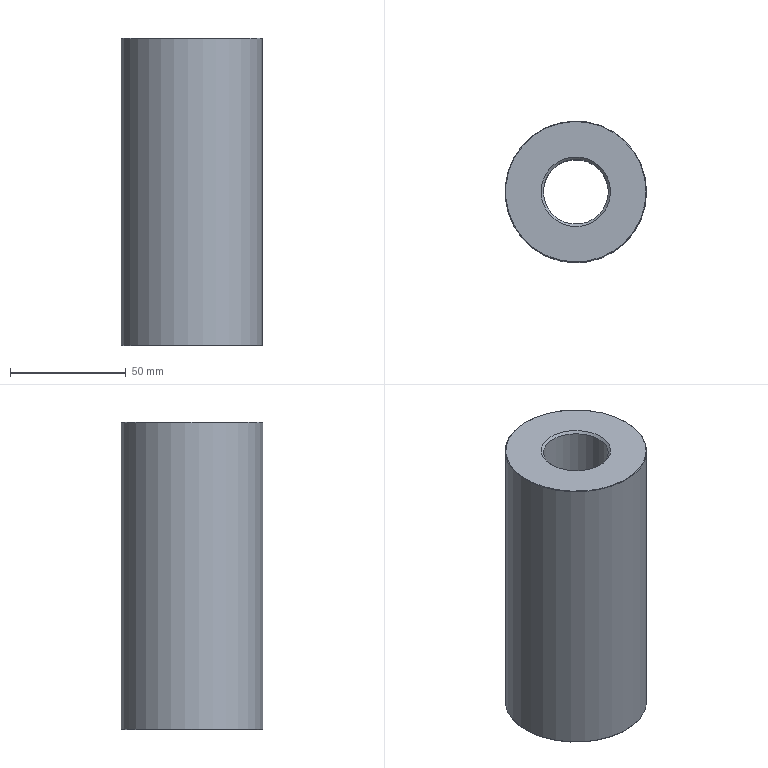Part | NX | features DATUM_CSYS 2, BLEND 1, CHAMFER 1, EXTRUDE 1, SKETCH 1 | 1 solid | 8 faces | box 61 x 61 x 132.5 mm | volume 305546 mm3 | cylinder 2 | plane 2 | cone 2 | torus 2 | commonest cylinder face diameters 28 x1 61 x1
STEP:
#1=CARTESIAN_POINT('',(30.5,0.,0.2));
#2=VERTEX_POINT('',#1);
#3=CARTESIAN_POINT('',(0.,0.,0.2));
#4=DIRECTION('',(0.,0.,1.));
#5=DIRECTION('',(1.,0.,0.));
#6=AXIS2_PLACEMENT_3D('',#3,#4,#5);
#7=CIRCLE('',#6,30.5);
#8=EDGE_CURVE('',#2,#2,#7,.T.);
#9=ORIENTED_EDGE('',*,*,#8,.T.);
#10=EDGE_LOOP('',(#9));
#11=FACE_BOUND('',#10,.T.);
#12=CARTESIAN_POINT('',(30.5,0.,132.3));
#13=VERTEX_POINT('',#12);
#14=CARTESIAN_POINT('',(0.,0.,132.3));
#15=DIRECTION('',(0.,0.,1.));
#16=DIRECTION('',(1.,0.,0.));
#17=AXIS2_PLACEMENT_3D('',#14,#15,#16);
#18=CIRCLE('',#17,30.5);
#19=EDGE_CURVE('',#13,#13,#18,.F.);
#20=ORIENTED_EDGE('',*,*,#19,.T.);
#21=EDGE_LOOP('',(#20));
#22=FACE_BOUND('',#21,.T.);
#23=CARTESIAN_POINT('',(0.,0.,132.5));
#24=DIRECTION('',(0.,0.,-1.));
#25=DIRECTION('',(-1.,0.,0.));
#26=AXIS2_PLACEMENT_3D('',#23,#24,#25);
#27=CYLINDRICAL_SURFACE('',#26,30.5);
#28=ADVANCED_FACE('',(#11,#22),#27,.T.);
#29=CARTESIAN_POINT('',(14.,0.,1.));
#30=VERTEX_POINT('',#29);
#31=CARTESIAN_POINT('',(0.,0.,1.));
#32=DIRECTION('',(0.,0.,1.));
#33=DIRECTION('',(1.,0.,0.));
#34=AXIS2_PLACEMENT_3D('',#31,#32,#33);
#35=CIRCLE('',#34,14.);
#36=EDGE_CURVE('',#30,#30,#35,.F.);
#37=ORIENTED_EDGE('',*,*,#36,.T.);
#38=EDGE_LOOP('',(#37));
#39=FACE_BOUND('',#38,.T.);
#40=CARTESIAN_POINT('',(14.,0.,131.5));
#41=VERTEX_POINT('',#40);
#42=CARTESIAN_POINT('',(0.,0.,131.5));
#43=DIRECTION('',(0.,0.,1.));
#44=DIRECTION('',(1.,0.,0.));
#45=AXIS2_PLACEMENT_3D('',#42,#43,#44);
#46=CIRCLE('',#45,14.);
#47=EDGE_CURVE('',#41,#41,#46,.T.);
#48=ORIENTED_EDGE('',*,*,#47,.T.);
#49=EDGE_LOOP('',(#48));
#50=FACE_BOUND('',#49,.T.);
#51=CARTESIAN_POINT('',(0.,0.,132.5));
#52=DIRECTION('',(0.,0.,-1.));
#53=DIRECTION('',(-1.,0.,0.));
#54=AXIS2_PLACEMENT_3D('',#51,#52,#53);
#55=CYLINDRICAL_SURFACE('',#54,14.);
#56=ADVANCED_FACE('',(#39,#50),#55,.F.);
#57=CARTESIAN_POINT('',(30.3,0.,132.5));
#58=VERTEX_POINT('',#57);
#59=CARTESIAN_POINT('',(0.,0.,132.5));
#60=DIRECTION('',(0.,0.,1.));
#61=DIRECTION('',(1.,0.,0.));
#62=AXIS2_PLACEMENT_3D('',#59,#60,#61);
#63=CIRCLE('',#62,30.3);
#64=EDGE_CURVE('',#58,#58,#63,.T.);
#65=ORIENTED_EDGE('',*,*,#64,.T.);
#66=EDGE_LOOP('',(#65));
#67=FACE_BOUND('',#66,.T.);
#68=CARTESIAN_POINT('',(15.,0.,132.5));
#69=VERTEX_POINT('',#68);
#70=CARTESIAN_POINT('',(0.,0.,132.5));
#71=DIRECTION('',(0.,0.,1.));
#72=DIRECTION('',(1.,0.,0.));
#73=AXIS2_PLACEMENT_3D('',#70,#71,#72);
#74=CIRCLE('',#73,15.);
#75=EDGE_CURVE('',#69,#69,#74,.F.);
#76=ORIENTED_EDGE('',*,*,#75,.T.);
#77=EDGE_LOOP('',(#76));
#78=FACE_BOUND('',#77,.T.);
#79=CARTESIAN_POINT('',(0.,0.,132.5));
#80=DIRECTION('',(0.,0.,1.));
#81=DIRECTION('',(1.,0.,0.));
#82=AXIS2_PLACEMENT_3D('',#79,#80,#81);
#83=PLANE('',#82);
#84=ADVANCED_FACE('',(#67,#78),#83,.T.);
#85=CARTESIAN_POINT('',(30.3,0.,0.));
#86=VERTEX_POINT('',#85);
#87=CARTESIAN_POINT('',(0.,0.,0.));
#88=DIRECTION('',(0.,0.,1.));
#89=DIRECTION('',(1.,0.,0.));
#90=AXIS2_PLACEMENT_3D('',#87,#88,#89);
#91=CIRCLE('',#90,30.3);
#92=EDGE_CURVE('',#86,#86,#91,.F.);
#93=ORIENTED_EDGE('',*,*,#92,.T.);
#94=EDGE_LOOP('',(#93));
#95=FACE_BOUND('',#94,.T.);
#96=CARTESIAN_POINT('',(15.,0.,0.));
#97=VERTEX_POINT('',#96);
#98=CARTESIAN_POINT('',(0.,0.,0.));
#99=DIRECTION('',(0.,0.,1.));
#100=DIRECTION('',(1.,0.,0.));
#101=AXIS2_PLACEMENT_3D('',#98,#99,#100);
#102=CIRCLE('',#101,15.);
#103=EDGE_CURVE('',#97,#97,#102,.T.);
#104=ORIENTED_EDGE('',*,*,#103,.T.);
#105=EDGE_LOOP('',(#104));
#106=FACE_BOUND('',#105,.T.);
#107=CARTESIAN_POINT('',(0.,0.,0.));
#108=DIRECTION('',(0.,0.,1.));
#109=DIRECTION('',(1.,0.,0.));
#110=AXIS2_PLACEMENT_3D('',#107,#108,#109);
#111=PLANE('',#110);
#112=ADVANCED_FACE('',(#95,#106),#111,.F.);
#113=ORIENTED_EDGE('',*,*,#36,.F.);
#114=EDGE_LOOP('',(#113));
#115=FACE_BOUND('',#114,.T.);
#116=ORIENTED_EDGE('',*,*,#103,.F.);
#117=EDGE_LOOP('',(#116));
#118=FACE_BOUND('',#117,.T.);
#119=CARTESIAN_POINT('',(0.,0.,0.));
#120=DIRECTION('',(0.,0.,-1.));
#121=DIRECTION('',(-1.,0.,0.));
#122=AXIS2_PLACEMENT_3D('',#119,#120,#121);
#123=CONICAL_SURFACE('',#122,15.,0.7854);
#124=ADVANCED_FACE('',(#115,#118),#123,.F.);
#125=ORIENTED_EDGE('',*,*,#75,.F.);
#126=EDGE_LOOP('',(#125));
#127=FACE_BOUND('',#126,.T.);
#128=ORIENTED_EDGE('',*,*,#47,.F.);
#129=EDGE_LOOP('',(#128));
#130=FACE_BOUND('',#129,.T.);
#131=CARTESIAN_POINT('',(0.,0.,131.5));
#132=DIRECTION('',(0.,0.,1.));
#133=DIRECTION('',(1.,0.,0.));
#134=AXIS2_PLACEMENT_3D('',#131,#132,#133);
#135=CONICAL_SURFACE('',#134,14.,0.7854);
#136=ADVANCED_FACE('',(#127,#130),#135,.F.);
#137=ORIENTED_EDGE('',*,*,#92,.F.);
#138=EDGE_LOOP('',(#137));
#139=FACE_BOUND('',#138,.T.);
#140=ORIENTED_EDGE('',*,*,#8,.F.);
#141=EDGE_LOOP('',(#140));
#142=FACE_BOUND('',#141,.T.);
#143=CARTESIAN_POINT('',(0.,0.,0.2));
#144=DIRECTION('',(0.,0.,1.));
#145=DIRECTION('',(1.,0.,0.));
#146=AXIS2_PLACEMENT_3D('',#143,#144,#145);
#147=TOROIDAL_SURFACE('',#146,30.3,0.2);
#148=ADVANCED_FACE('',(#139,#142),#147,.T.);
#149=ORIENTED_EDGE('',*,*,#19,.F.);
#150=EDGE_LOOP('',(#149));
#151=FACE_BOUND('',#150,.T.);
#152=ORIENTED_EDGE('',*,*,#64,.F.);
#153=EDGE_LOOP('',(#152));
#154=FACE_BOUND('',#153,.T.);
#155=CARTESIAN_POINT('',(0.,0.,132.3));
#156=DIRECTION('',(0.,0.,1.));
#157=DIRECTION('',(1.,0.,0.));
#158=AXIS2_PLACEMENT_3D('',#155,#156,#157);
#159=TOROIDAL_SURFACE('',#158,30.3,0.2);
#160=ADVANCED_FACE('',(#151,#154),#159,.T.);
#161=CLOSED_SHELL('',(#28,#56,#84,#112,#124,#136,#148,#160));
#162=MANIFOLD_SOLID_BREP('',#161);
#163=(LENGTH_UNIT()NAMED_UNIT(*)SI_UNIT(.MILLI.,.METRE.));
#164=UNCERTAINTY_MEASURE_WITH_UNIT(LENGTH_MEASURE(0.00001),#163,'','');
#165=(NAMED_UNIT(*)PLANE_ANGLE_UNIT()SI_UNIT($,.RADIAN.));
#166=(NAMED_UNIT(*)SI_UNIT($,.STERADIAN.)SOLID_ANGLE_UNIT());
#167=(GEOMETRIC_REPRESENTATION_CONTEXT(3)GLOBAL_UNCERTAINTY_ASSIGNED_CONTEXT((#164))GLOBAL_UNIT_ASSIGNED_CONTEXT((#163,#165,#166))REPRESENTATION_CONTEXT('',''));
#168=ADVANCED_BREP_SHAPE_REPRESENTATION('',(#162),#167);